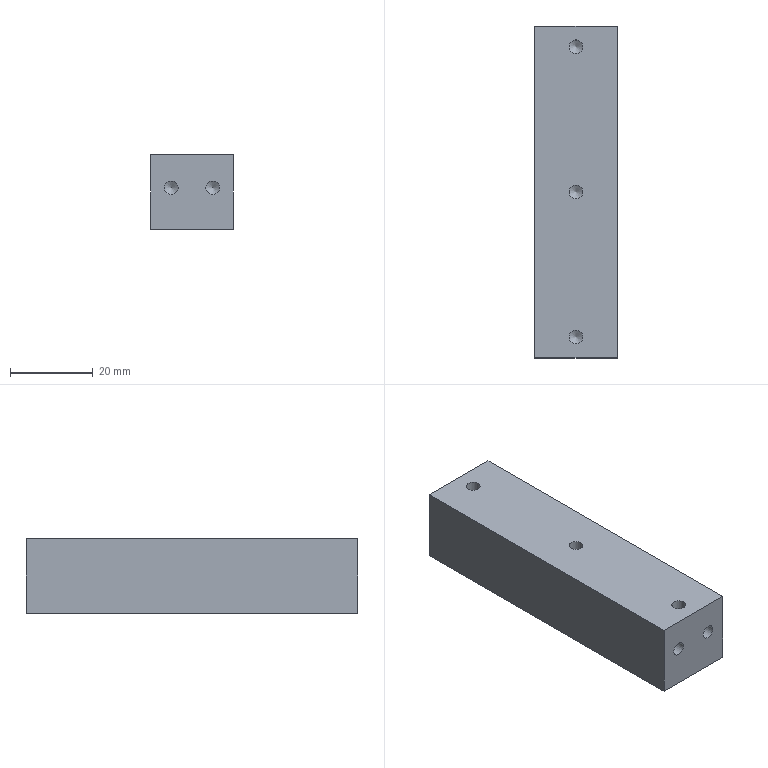Part | NX | 1 solid | 24 faces | box 20 x 80 x 18 mm | volume 27997 mm3 | cone 9 | cylinder 9 | plane 6 | commonest cylinder face diameters 3.3 x9
STEP:
#1=CARTESIAN_POINT('',(10.,-40.,0.));
#2=VERTEX_POINT('',#1);
#3=CARTESIAN_POINT('',(10.,40.,0.));
#4=VERTEX_POINT('',#3);
#5=CARTESIAN_POINT('',(10.,40.,0.));
#6=DIRECTION('',(0.,1.,0.));
#7=VECTOR('',#6,1000.);
#8=LINE('',#5,#7);
#9=EDGE_CURVE('',#2,#4,#8,.T.);
#10=ORIENTED_EDGE('',*,*,#9,.T.);
#11=CARTESIAN_POINT('',(10.,40.,18.));
#12=VERTEX_POINT('',#11);
#13=CARTESIAN_POINT('',(10.,40.,18.));
#14=DIRECTION('',(0.,0.,-1.));
#15=VECTOR('',#14,1000.);
#16=LINE('',#13,#15);
#17=EDGE_CURVE('',#12,#4,#16,.T.);
#18=ORIENTED_EDGE('',*,*,#17,.F.);
#19=CARTESIAN_POINT('',(10.,-40.,18.));
#20=VERTEX_POINT('',#19);
#21=CARTESIAN_POINT('',(10.,40.,18.));
#22=DIRECTION('',(0.,1.,0.));
#23=VECTOR('',#22,1000.);
#24=LINE('',#21,#23);
#25=EDGE_CURVE('',#20,#12,#24,.T.);
#26=ORIENTED_EDGE('',*,*,#25,.F.);
#27=CARTESIAN_POINT('',(10.,-40.,18.));
#28=DIRECTION('',(0.,0.,-1.));
#29=VECTOR('',#28,1000.);
#30=LINE('',#27,#29);
#31=EDGE_CURVE('',#20,#2,#30,.T.);
#32=ORIENTED_EDGE('',*,*,#31,.T.);
#33=EDGE_LOOP('',(#10,#18,#26,#32));
#34=FACE_BOUND('',#33,.T.);
#35=CARTESIAN_POINT('',(10.,40.,18.));
#36=DIRECTION('',(-1.,0.,0.));
#37=DIRECTION('',(0.,-1.,0.));
#38=AXIS2_PLACEMENT_3D('',#35,#36,#37);
#39=PLANE('',#38);
#40=ADVANCED_FACE('',(#34),#39,.F.);
#41=CARTESIAN_POINT('',(-5.,40.,11.65));
#42=VERTEX_POINT('',#41);
#43=CARTESIAN_POINT('',(-5.,40.,10.));
#44=DIRECTION('',(0.,1.,0.));
#45=DIRECTION('',(0.,0.,1.));
#46=AXIS2_PLACEMENT_3D('',#43,#44,#45);
#47=CIRCLE('',#46,1.65);
#48=EDGE_CURVE('',#42,#42,#47,.T.);
#49=ORIENTED_EDGE('',*,*,#48,.F.);
#50=EDGE_LOOP('',(#49));
#51=FACE_BOUND('',#50,.T.);
#52=CARTESIAN_POINT('',(5.,40.,11.65));
#53=VERTEX_POINT('',#52);
#54=CARTESIAN_POINT('',(5.,40.,10.));
#55=DIRECTION('',(0.,1.,0.));
#56=DIRECTION('',(0.,0.,1.));
#57=AXIS2_PLACEMENT_3D('',#54,#55,#56);
#58=CIRCLE('',#57,1.65);
#59=EDGE_CURVE('',#53,#53,#58,.T.);
#60=ORIENTED_EDGE('',*,*,#59,.F.);
#61=EDGE_LOOP('',(#60));
#62=FACE_BOUND('',#61,.T.);
#63=CARTESIAN_POINT('',(-10.,40.,0.));
#64=VERTEX_POINT('',#63);
#65=CARTESIAN_POINT('',(-10.,40.,0.));
#66=DIRECTION('',(-1.,0.,0.));
#67=VECTOR('',#66,1000.);
#68=LINE('',#65,#67);
#69=EDGE_CURVE('',#4,#64,#68,.T.);
#70=ORIENTED_EDGE('',*,*,#69,.T.);
#71=CARTESIAN_POINT('',(-10.,40.,18.));
#72=VERTEX_POINT('',#71);
#73=CARTESIAN_POINT('',(-10.,40.,18.));
#74=DIRECTION('',(0.,0.,-1.));
#75=VECTOR('',#74,1000.);
#76=LINE('',#73,#75);
#77=EDGE_CURVE('',#72,#64,#76,.T.);
#78=ORIENTED_EDGE('',*,*,#77,.F.);
#79=CARTESIAN_POINT('',(-10.,40.,18.));
#80=DIRECTION('',(-1.,0.,0.));
#81=VECTOR('',#80,1000.);
#82=LINE('',#79,#81);
#83=EDGE_CURVE('',#12,#72,#82,.T.);
#84=ORIENTED_EDGE('',*,*,#83,.F.);
#85=ORIENTED_EDGE('',*,*,#17,.T.);
#86=EDGE_LOOP('',(#70,#78,#84,#85));
#87=FACE_BOUND('',#86,.T.);
#88=CARTESIAN_POINT('',(-10.,40.,18.));
#89=DIRECTION('',(0.,-1.,0.));
#90=DIRECTION('',(0.,0.,-1.));
#91=AXIS2_PLACEMENT_3D('',#88,#89,#90);
#92=PLANE('',#91);
#93=ADVANCED_FACE('',(#51,#62,#87),#92,.F.);
#94=CARTESIAN_POINT('',(-10.,-40.,0.));
#95=VERTEX_POINT('',#94);
#96=CARTESIAN_POINT('',(-10.,40.,0.));
#97=DIRECTION('',(0.,-1.,0.));
#98=VECTOR('',#97,1000.);
#99=LINE('',#96,#98);
#100=EDGE_CURVE('',#64,#95,#99,.T.);
#101=ORIENTED_EDGE('',*,*,#100,.T.);
#102=CARTESIAN_POINT('',(-10.,-40.,18.));
#103=VERTEX_POINT('',#102);
#104=CARTESIAN_POINT('',(-10.,-40.,18.));
#105=DIRECTION('',(0.,0.,-1.));
#106=VECTOR('',#105,1000.);
#107=LINE('',#104,#106);
#108=EDGE_CURVE('',#103,#95,#107,.T.);
#109=ORIENTED_EDGE('',*,*,#108,.F.);
#110=CARTESIAN_POINT('',(-10.,40.,18.));
#111=DIRECTION('',(0.,-1.,0.));
#112=VECTOR('',#111,1000.);
#113=LINE('',#110,#112);
#114=EDGE_CURVE('',#72,#103,#113,.T.);
#115=ORIENTED_EDGE('',*,*,#114,.F.);
#116=ORIENTED_EDGE('',*,*,#77,.T.);
#117=EDGE_LOOP('',(#101,#109,#115,#116));
#118=FACE_BOUND('',#117,.T.);
#119=CARTESIAN_POINT('',(-10.,40.,18.));
#120=DIRECTION('',(1.,0.,0.));
#121=DIRECTION('',(0.,1.,0.));
#122=AXIS2_PLACEMENT_3D('',#119,#120,#121);
#123=PLANE('',#122);
#124=ADVANCED_FACE('',(#118),#123,.F.);
#125=CARTESIAN_POINT('',(-5.,-40.,8.35));
#126=VERTEX_POINT('',#125);
#127=CARTESIAN_POINT('',(-5.,-40.,10.));
#128=DIRECTION('',(0.,-1.,0.));
#129=DIRECTION('',(0.,0.,-1.));
#130=AXIS2_PLACEMENT_3D('',#127,#128,#129);
#131=CIRCLE('',#130,1.65);
#132=EDGE_CURVE('',#126,#126,#131,.T.);
#133=ORIENTED_EDGE('',*,*,#132,.F.);
#134=EDGE_LOOP('',(#133));
#135=FACE_BOUND('',#134,.T.);
#136=CARTESIAN_POINT('',(5.,-40.,8.35));
#137=VERTEX_POINT('',#136);
#138=CARTESIAN_POINT('',(5.,-40.,10.));
#139=DIRECTION('',(0.,-1.,0.));
#140=DIRECTION('',(0.,0.,-1.));
#141=AXIS2_PLACEMENT_3D('',#138,#139,#140);
#142=CIRCLE('',#141,1.65);
#143=EDGE_CURVE('',#137,#137,#142,.T.);
#144=ORIENTED_EDGE('',*,*,#143,.F.);
#145=EDGE_LOOP('',(#144));
#146=FACE_BOUND('',#145,.T.);
#147=CARTESIAN_POINT('',(-10.,-40.,0.));
#148=DIRECTION('',(1.,0.,0.));
#149=VECTOR('',#148,1000.);
#150=LINE('',#147,#149);
#151=EDGE_CURVE('',#95,#2,#150,.T.);
#152=ORIENTED_EDGE('',*,*,#151,.T.);
#153=ORIENTED_EDGE('',*,*,#31,.F.);
#154=CARTESIAN_POINT('',(-10.,-40.,18.));
#155=DIRECTION('',(1.,0.,0.));
#156=VECTOR('',#155,1000.);
#157=LINE('',#154,#156);
#158=EDGE_CURVE('',#103,#20,#157,.T.);
#159=ORIENTED_EDGE('',*,*,#158,.F.);
#160=ORIENTED_EDGE('',*,*,#108,.T.);
#161=EDGE_LOOP('',(#152,#153,#159,#160));
#162=FACE_BOUND('',#161,.T.);
#163=CARTESIAN_POINT('',(-10.,-40.,18.));
#164=DIRECTION('',(0.,1.,0.));
#165=DIRECTION('',(-1.,0.,0.));
#166=AXIS2_PLACEMENT_3D('',#163,#164,#165);
#167=PLANE('',#166);
#168=ADVANCED_FACE('',(#135,#146,#162),#167,.F.);
#169=CARTESIAN_POINT('',(1.65,35.,18.));
#170=VERTEX_POINT('',#169);
#171=CARTESIAN_POINT('',(0.,35.,18.));
#172=DIRECTION('',(0.,0.,1.));
#173=DIRECTION('',(1.,0.,0.));
#174=AXIS2_PLACEMENT_3D('',#171,#172,#173);
#175=CIRCLE('',#174,1.65);
#176=EDGE_CURVE('',#170,#170,#175,.T.);
#177=ORIENTED_EDGE('',*,*,#176,.F.);
#178=EDGE_LOOP('',(#177));
#179=FACE_BOUND('',#178,.T.);
#180=CARTESIAN_POINT('',(1.65,-35.,18.));
#181=VERTEX_POINT('',#180);
#182=CARTESIAN_POINT('',(0.,-35.,18.));
#183=DIRECTION('',(0.,0.,1.));
#184=DIRECTION('',(1.,0.,0.));
#185=AXIS2_PLACEMENT_3D('',#182,#183,#184);
#186=CIRCLE('',#185,1.65);
#187=EDGE_CURVE('',#181,#181,#186,.T.);
#188=ORIENTED_EDGE('',*,*,#187,.F.);
#189=EDGE_LOOP('',(#188));
#190=FACE_BOUND('',#189,.T.);
#191=CARTESIAN_POINT('',(1.65,0.,18.));
#192=VERTEX_POINT('',#191);
#193=CARTESIAN_POINT('',(0.,0.,18.));
#194=DIRECTION('',(0.,0.,1.));
#195=DIRECTION('',(1.,0.,0.));
#196=AXIS2_PLACEMENT_3D('',#193,#194,#195);
#197=CIRCLE('',#196,1.65);
#198=EDGE_CURVE('',#192,#192,#197,.T.);
#199=ORIENTED_EDGE('',*,*,#198,.F.);
#200=EDGE_LOOP('',(#199));
#201=FACE_BOUND('',#200,.T.);
#202=ORIENTED_EDGE('',*,*,#25,.T.);
#203=ORIENTED_EDGE('',*,*,#83,.T.);
#204=ORIENTED_EDGE('',*,*,#114,.T.);
#205=ORIENTED_EDGE('',*,*,#158,.T.);
#206=EDGE_LOOP('',(#202,#203,#204,#205));
#207=FACE_BOUND('',#206,.T.);
#208=CARTESIAN_POINT('',(0.,0.,18.));
#209=DIRECTION('',(0.,0.,1.));
#210=DIRECTION('',(1.,0.,0.));
#211=AXIS2_PLACEMENT_3D('',#208,#209,#210);
#212=PLANE('',#211);
#213=ADVANCED_FACE('',(#179,#190,#201,#207),#212,.T.);
#214=CARTESIAN_POINT('',(-1.65,30.,0.));
#215=VERTEX_POINT('',#214);
#216=CARTESIAN_POINT('',(0.,30.,0.));
#217=DIRECTION('',(0.,0.,-1.));
#218=DIRECTION('',(-1.,0.,0.));
#219=AXIS2_PLACEMENT_3D('',#216,#217,#218);
#220=CIRCLE('',#219,1.65);
#221=EDGE_CURVE('',#215,#215,#220,.T.);
#222=ORIENTED_EDGE('',*,*,#221,.F.);
#223=EDGE_LOOP('',(#222));
#224=FACE_BOUND('',#223,.T.);
#225=CARTESIAN_POINT('',(-1.65,-30.,0.));
#226=VERTEX_POINT('',#225);
#227=CARTESIAN_POINT('',(0.,-30.,0.));
#228=DIRECTION('',(0.,0.,-1.));
#229=DIRECTION('',(-1.,0.,0.));
#230=AXIS2_PLACEMENT_3D('',#227,#228,#229);
#231=CIRCLE('',#230,1.65);
#232=EDGE_CURVE('',#226,#226,#231,.T.);
#233=ORIENTED_EDGE('',*,*,#232,.F.);
#234=EDGE_LOOP('',(#233));
#235=FACE_BOUND('',#234,.T.);
#236=ORIENTED_EDGE('',*,*,#9,.F.);
#237=ORIENTED_EDGE('',*,*,#151,.F.);
#238=ORIENTED_EDGE('',*,*,#100,.F.);
#239=ORIENTED_EDGE('',*,*,#69,.F.);
#240=EDGE_LOOP('',(#236,#237,#238,#239));
#241=FACE_BOUND('',#240,.T.);
#242=CARTESIAN_POINT('',(0.,0.,0.));
#243=DIRECTION('',(0.,0.,1.));
#244=DIRECTION('',(1.,0.,0.));
#245=AXIS2_PLACEMENT_3D('',#242,#243,#244);
#246=PLANE('',#245);
#247=ADVANCED_FACE('',(#224,#235,#241),#246,.F.);
#248=CARTESIAN_POINT('',(0.,0.,6.909));
#249=VERTEX_POINT('',#248);
#250=VERTEX_LOOP('',#249);
#251=FACE_BOUND('',#250,.T.);
#252=CARTESIAN_POINT('',(1.65,0.,7.9));
#253=VERTEX_POINT('',#252);
#254=CARTESIAN_POINT('',(0.,0.,7.9));
#255=DIRECTION('',(0.,0.,1.));
#256=DIRECTION('',(1.,0.,0.));
#257=AXIS2_PLACEMENT_3D('',#254,#255,#256);
#258=CIRCLE('',#257,1.65);
#259=EDGE_CURVE('',#253,#253,#258,.T.);
#260=ORIENTED_EDGE('',*,*,#259,.T.);
#261=EDGE_LOOP('',(#260));
#262=FACE_BOUND('',#261,.T.);
#263=CARTESIAN_POINT('',(0.,0.,7.9));
#264=DIRECTION('',(0.,0.,1.));
#265=DIRECTION('',(1.,0.,0.));
#266=AXIS2_PLACEMENT_3D('',#263,#264,#265);
#267=CONICAL_SURFACE('',#266,1.65,1.03);
#268=ADVANCED_FACE('',(#251,#262),#267,.F.);
#269=ORIENTED_EDGE('',*,*,#259,.F.);
#270=EDGE_LOOP('',(#269));
#271=FACE_BOUND('',#270,.T.);
#272=ORIENTED_EDGE('',*,*,#198,.T.);
#273=EDGE_LOOP('',(#272));
#274=FACE_BOUND('',#273,.T.);
#275=CARTESIAN_POINT('',(0.,0.,18.));
#276=DIRECTION('',(0.,0.,1.));
#277=DIRECTION('',(1.,0.,0.));
#278=AXIS2_PLACEMENT_3D('',#275,#276,#277);
#279=CYLINDRICAL_SURFACE('',#278,1.65);
#280=ADVANCED_FACE('',(#271,#274),#279,.F.);
#281=CARTESIAN_POINT('',(0.,-35.,6.909));
#282=VERTEX_POINT('',#281);
#283=VERTEX_LOOP('',#282);
#284=FACE_BOUND('',#283,.T.);
#285=CARTESIAN_POINT('',(1.65,-35.,7.9));
#286=VERTEX_POINT('',#285);
#287=CARTESIAN_POINT('',(0.,-35.,7.9));
#288=DIRECTION('',(0.,0.,1.));
#289=DIRECTION('',(1.,0.,0.));
#290=AXIS2_PLACEMENT_3D('',#287,#288,#289);
#291=CIRCLE('',#290,1.65);
#292=EDGE_CURVE('',#286,#286,#291,.T.);
#293=ORIENTED_EDGE('',*,*,#292,.T.);
#294=EDGE_LOOP('',(#293));
#295=FACE_BOUND('',#294,.T.);
#296=CARTESIAN_POINT('',(0.,-35.,7.9));
#297=DIRECTION('',(0.,0.,1.));
#298=DIRECTION('',(1.,0.,0.));
#299=AXIS2_PLACEMENT_3D('',#296,#297,#298);
#300=CONICAL_SURFACE('',#299,1.65,1.03);
#301=ADVANCED_FACE('',(#284,#295),#300,.F.);
#302=ORIENTED_EDGE('',*,*,#292,.F.);
#303=EDGE_LOOP('',(#302));
#304=FACE_BOUND('',#303,.T.);
#305=ORIENTED_EDGE('',*,*,#187,.T.);
#306=EDGE_LOOP('',(#305));
#307=FACE_BOUND('',#306,.T.);
#308=CARTESIAN_POINT('',(0.,-35.,18.));
#309=DIRECTION('',(0.,0.,1.));
#310=DIRECTION('',(1.,0.,0.));
#311=AXIS2_PLACEMENT_3D('',#308,#309,#310);
#312=CYLINDRICAL_SURFACE('',#311,1.65);
#313=ADVANCED_FACE('',(#304,#307),#312,.F.);
#314=CARTESIAN_POINT('',(0.,35.,6.909));
#315=VERTEX_POINT('',#314);
#316=VERTEX_LOOP('',#315);
#317=FACE_BOUND('',#316,.T.);
#318=CARTESIAN_POINT('',(1.65,35.,7.9));
#319=VERTEX_POINT('',#318);
#320=CARTESIAN_POINT('',(0.,35.,7.9));
#321=DIRECTION('',(0.,0.,1.));
#322=DIRECTION('',(1.,0.,0.));
#323=AXIS2_PLACEMENT_3D('',#320,#321,#322);
#324=CIRCLE('',#323,1.65);
#325=EDGE_CURVE('',#319,#319,#324,.T.);
#326=ORIENTED_EDGE('',*,*,#325,.T.);
#327=EDGE_LOOP('',(#326));
#328=FACE_BOUND('',#327,.T.);
#329=CARTESIAN_POINT('',(0.,35.,7.9));
#330=DIRECTION('',(0.,0.,1.));
#331=DIRECTION('',(1.,0.,0.));
#332=AXIS2_PLACEMENT_3D('',#329,#330,#331);
#333=CONICAL_SURFACE('',#332,1.65,1.03);
#334=ADVANCED_FACE('',(#317,#328),#333,.F.);
#335=ORIENTED_EDGE('',*,*,#325,.F.);
#336=EDGE_LOOP('',(#335));
#337=FACE_BOUND('',#336,.T.);
#338=ORIENTED_EDGE('',*,*,#176,.T.);
#339=EDGE_LOOP('',(#338));
#340=FACE_BOUND('',#339,.T.);
#341=CARTESIAN_POINT('',(0.,35.,18.));
#342=DIRECTION('',(0.,0.,1.));
#343=DIRECTION('',(1.,0.,0.));
#344=AXIS2_PLACEMENT_3D('',#341,#342,#343);
#345=CYLINDRICAL_SURFACE('',#344,1.65);
#346=ADVANCED_FACE('',(#337,#340),#345,.F.);
#347=CARTESIAN_POINT('',(0.,-30.,11.091));
#348=VERTEX_POINT('',#347);
#349=VERTEX_LOOP('',#348);
#350=FACE_BOUND('',#349,.T.);
#351=CARTESIAN_POINT('',(-1.65,-30.,10.1));
#352=VERTEX_POINT('',#351);
#353=CARTESIAN_POINT('',(0.,-30.,10.1));
#354=DIRECTION('',(0.,0.,-1.));
#355=DIRECTION('',(-1.,0.,0.));
#356=AXIS2_PLACEMENT_3D('',#353,#354,#355);
#357=CIRCLE('',#356,1.65);
#358=EDGE_CURVE('',#352,#352,#357,.T.);
#359=ORIENTED_EDGE('',*,*,#358,.T.);
#360=EDGE_LOOP('',(#359));
#361=FACE_BOUND('',#360,.T.);
#362=CARTESIAN_POINT('',(0.,-30.,10.1));
#363=DIRECTION('',(0.,0.,-1.));
#364=DIRECTION('',(-1.,0.,0.));
#365=AXIS2_PLACEMENT_3D('',#362,#363,#364);
#366=CONICAL_SURFACE('',#365,1.65,1.03);
#367=ADVANCED_FACE('',(#350,#361),#366,.F.);
#368=ORIENTED_EDGE('',*,*,#358,.F.);
#369=EDGE_LOOP('',(#368));
#370=FACE_BOUND('',#369,.T.);
#371=ORIENTED_EDGE('',*,*,#232,.T.);
#372=EDGE_LOOP('',(#371));
#373=FACE_BOUND('',#372,.T.);
#374=CARTESIAN_POINT('',(0.,-30.,0.));
#375=DIRECTION('',(0.,0.,-1.));
#376=DIRECTION('',(-1.,0.,0.));
#377=AXIS2_PLACEMENT_3D('',#374,#375,#376);
#378=CYLINDRICAL_SURFACE('',#377,1.65);
#379=ADVANCED_FACE('',(#370,#373),#378,.F.);
#380=CARTESIAN_POINT('',(0.,30.,11.091));
#381=VERTEX_POINT('',#380);
#382=VERTEX_LOOP('',#381);
#383=FACE_BOUND('',#382,.T.);
#384=CARTESIAN_POINT('',(-1.65,30.,10.1));
#385=VERTEX_POINT('',#384);
#386=CARTESIAN_POINT('',(0.,30.,10.1));
#387=DIRECTION('',(0.,0.,-1.));
#388=DIRECTION('',(-1.,0.,0.));
#389=AXIS2_PLACEMENT_3D('',#386,#387,#388);
#390=CIRCLE('',#389,1.65);
#391=EDGE_CURVE('',#385,#385,#390,.T.);
#392=ORIENTED_EDGE('',*,*,#391,.T.);
#393=EDGE_LOOP('',(#392));
#394=FACE_BOUND('',#393,.T.);
#395=CARTESIAN_POINT('',(0.,30.,10.1));
#396=DIRECTION('',(0.,0.,-1.));
#397=DIRECTION('',(-1.,0.,0.));
#398=AXIS2_PLACEMENT_3D('',#395,#396,#397);
#399=CONICAL_SURFACE('',#398,1.65,1.03);
#400=ADVANCED_FACE('',(#383,#394),#399,.F.);
#401=ORIENTED_EDGE('',*,*,#391,.F.);
#402=EDGE_LOOP('',(#401));
#403=FACE_BOUND('',#402,.T.);
#404=ORIENTED_EDGE('',*,*,#221,.T.);
#405=EDGE_LOOP('',(#404));
#406=FACE_BOUND('',#405,.T.);
#407=CARTESIAN_POINT('',(0.,30.,0.));
#408=DIRECTION('',(0.,0.,-1.));
#409=DIRECTION('',(-1.,0.,0.));
#410=AXIS2_PLACEMENT_3D('',#407,#408,#409);
#411=CYLINDRICAL_SURFACE('',#410,1.65);
#412=ADVANCED_FACE('',(#403,#406),#411,.F.);
#413=CARTESIAN_POINT('',(5.,28.909,10.));
#414=VERTEX_POINT('',#413);
#415=VERTEX_LOOP('',#414);
#416=FACE_BOUND('',#415,.T.);
#417=CARTESIAN_POINT('',(5.,29.9,11.65));
#418=VERTEX_POINT('',#417);
#419=CARTESIAN_POINT('',(5.,29.9,10.));
#420=DIRECTION('',(0.,1.,0.));
#421=DIRECTION('',(0.,0.,1.));
#422=AXIS2_PLACEMENT_3D('',#419,#420,#421);
#423=CIRCLE('',#422,1.65);
#424=EDGE_CURVE('',#418,#418,#423,.T.);
#425=ORIENTED_EDGE('',*,*,#424,.T.);
#426=EDGE_LOOP('',(#425));
#427=FACE_BOUND('',#426,.T.);
#428=CARTESIAN_POINT('',(5.,29.9,10.));
#429=DIRECTION('',(0.,1.,0.));
#430=DIRECTION('',(0.,0.,1.));
#431=AXIS2_PLACEMENT_3D('',#428,#429,#430);
#432=CONICAL_SURFACE('',#431,1.65,1.03);
#433=ADVANCED_FACE('',(#416,#427),#432,.F.);
#434=ORIENTED_EDGE('',*,*,#424,.F.);
#435=EDGE_LOOP('',(#434));
#436=FACE_BOUND('',#435,.T.);
#437=ORIENTED_EDGE('',*,*,#59,.T.);
#438=EDGE_LOOP('',(#437));
#439=FACE_BOUND('',#438,.T.);
#440=CARTESIAN_POINT('',(5.,40.,10.));
#441=DIRECTION('',(0.,1.,0.));
#442=DIRECTION('',(0.,0.,1.));
#443=AXIS2_PLACEMENT_3D('',#440,#441,#442);
#444=CYLINDRICAL_SURFACE('',#443,1.65);
#445=ADVANCED_FACE('',(#436,#439),#444,.F.);
#446=CARTESIAN_POINT('',(-5.,28.909,10.));
#447=VERTEX_POINT('',#446);
#448=VERTEX_LOOP('',#447);
#449=FACE_BOUND('',#448,.T.);
#450=CARTESIAN_POINT('',(-5.,29.9,11.65));
#451=VERTEX_POINT('',#450);
#452=CARTESIAN_POINT('',(-5.,29.9,10.));
#453=DIRECTION('',(0.,1.,0.));
#454=DIRECTION('',(0.,0.,1.));
#455=AXIS2_PLACEMENT_3D('',#452,#453,#454);
#456=CIRCLE('',#455,1.65);
#457=EDGE_CURVE('',#451,#451,#456,.T.);
#458=ORIENTED_EDGE('',*,*,#457,.T.);
#459=EDGE_LOOP('',(#458));
#460=FACE_BOUND('',#459,.T.);
#461=CARTESIAN_POINT('',(-5.,29.9,10.));
#462=DIRECTION('',(0.,1.,0.));
#463=DIRECTION('',(0.,0.,1.));
#464=AXIS2_PLACEMENT_3D('',#461,#462,#463);
#465=CONICAL_SURFACE('',#464,1.65,1.03);
#466=ADVANCED_FACE('',(#449,#460),#465,.F.);
#467=ORIENTED_EDGE('',*,*,#457,.F.);
#468=EDGE_LOOP('',(#467));
#469=FACE_BOUND('',#468,.T.);
#470=ORIENTED_EDGE('',*,*,#48,.T.);
#471=EDGE_LOOP('',(#470));
#472=FACE_BOUND('',#471,.T.);
#473=CARTESIAN_POINT('',(-5.,40.,10.));
#474=DIRECTION('',(0.,1.,0.));
#475=DIRECTION('',(0.,0.,1.));
#476=AXIS2_PLACEMENT_3D('',#473,#474,#475);
#477=CYLINDRICAL_SURFACE('',#476,1.65);
#478=ADVANCED_FACE('',(#469,#472),#477,.F.);
#479=CARTESIAN_POINT('',(5.,-28.909,10.));
#480=VERTEX_POINT('',#479);
#481=VERTEX_LOOP('',#480);
#482=FACE_BOUND('',#481,.T.);
#483=CARTESIAN_POINT('',(5.,-29.9,8.35));
#484=VERTEX_POINT('',#483);
#485=CARTESIAN_POINT('',(5.,-29.9,10.));
#486=DIRECTION('',(0.,-1.,0.));
#487=DIRECTION('',(0.,0.,-1.));
#488=AXIS2_PLACEMENT_3D('',#485,#486,#487);
#489=CIRCLE('',#488,1.65);
#490=EDGE_CURVE('',#484,#484,#489,.T.);
#491=ORIENTED_EDGE('',*,*,#490,.T.);
#492=EDGE_LOOP('',(#491));
#493=FACE_BOUND('',#492,.T.);
#494=CARTESIAN_POINT('',(5.,-29.9,10.));
#495=DIRECTION('',(0.,-1.,0.));
#496=DIRECTION('',(0.,0.,-1.));
#497=AXIS2_PLACEMENT_3D('',#494,#495,#496);
#498=CONICAL_SURFACE('',#497,1.65,1.03);
#499=ADVANCED_FACE('',(#482,#493),#498,.F.);
#500=ORIENTED_EDGE('',*,*,#490,.F.);
#501=EDGE_LOOP('',(#500));
#502=FACE_BOUND('',#501,.T.);
#503=ORIENTED_EDGE('',*,*,#143,.T.);
#504=EDGE_LOOP('',(#503));
#505=FACE_BOUND('',#504,.T.);
#506=CARTESIAN_POINT('',(5.,-40.,10.));
#507=DIRECTION('',(0.,-1.,0.));
#508=DIRECTION('',(0.,0.,-1.));
#509=AXIS2_PLACEMENT_3D('',#506,#507,#508);
#510=CYLINDRICAL_SURFACE('',#509,1.65);
#511=ADVANCED_FACE('',(#502,#505),#510,.F.);
#512=CARTESIAN_POINT('',(-5.,-28.909,10.));
#513=VERTEX_POINT('',#512);
#514=VERTEX_LOOP('',#513);
#515=FACE_BOUND('',#514,.T.);
#516=CARTESIAN_POINT('',(-5.,-29.9,8.35));
#517=VERTEX_POINT('',#516);
#518=CARTESIAN_POINT('',(-5.,-29.9,10.));
#519=DIRECTION('',(0.,-1.,0.));
#520=DIRECTION('',(0.,0.,-1.));
#521=AXIS2_PLACEMENT_3D('',#518,#519,#520);
#522=CIRCLE('',#521,1.65);
#523=EDGE_CURVE('',#517,#517,#522,.T.);
#524=ORIENTED_EDGE('',*,*,#523,.T.);
#525=EDGE_LOOP('',(#524));
#526=FACE_BOUND('',#525,.T.);
#527=CARTESIAN_POINT('',(-5.,-29.9,10.));
#528=DIRECTION('',(0.,-1.,0.));
#529=DIRECTION('',(0.,0.,-1.));
#530=AXIS2_PLACEMENT_3D('',#527,#528,#529);
#531=CONICAL_SURFACE('',#530,1.65,1.03);
#532=ADVANCED_FACE('',(#515,#526),#531,.F.);
#533=ORIENTED_EDGE('',*,*,#523,.F.);
#534=EDGE_LOOP('',(#533));
#535=FACE_BOUND('',#534,.T.);
#536=ORIENTED_EDGE('',*,*,#132,.T.);
#537=EDGE_LOOP('',(#536));
#538=FACE_BOUND('',#537,.T.);
#539=CARTESIAN_POINT('',(-5.,-40.,10.));
#540=DIRECTION('',(0.,-1.,0.));
#541=DIRECTION('',(0.,0.,-1.));
#542=AXIS2_PLACEMENT_3D('',#539,#540,#541);
#543=CYLINDRICAL_SURFACE('',#542,1.65);
#544=ADVANCED_FACE('',(#535,#538),#543,.F.);
#545=CLOSED_SHELL('',(#40,#93,#124,#168,#213,#247,#268,#280,#301,#313,#334,#346,#367,#379,#400,#412,#433,#445,#466,#478,#499,#511,#532,#544));
#546=MANIFOLD_SOLID_BREP('',#545);
#547=(LENGTH_UNIT()NAMED_UNIT(*)SI_UNIT(.MILLI.,.METRE.));
#548=UNCERTAINTY_MEASURE_WITH_UNIT(LENGTH_MEASURE(0.00001),#547,'','');
#549=(NAMED_UNIT(*)PLANE_ANGLE_UNIT()SI_UNIT($,.RADIAN.));
#550=(NAMED_UNIT(*)SI_UNIT($,.STERADIAN.)SOLID_ANGLE_UNIT());
#551=(GEOMETRIC_REPRESENTATION_CONTEXT(3)GLOBAL_UNCERTAINTY_ASSIGNED_CONTEXT((#548))GLOBAL_UNIT_ASSIGNED_CONTEXT((#547,#549,#550))REPRESENTATION_CONTEXT('',''));
#552=ADVANCED_BREP_SHAPE_REPRESENTATION('',(#546),#551);